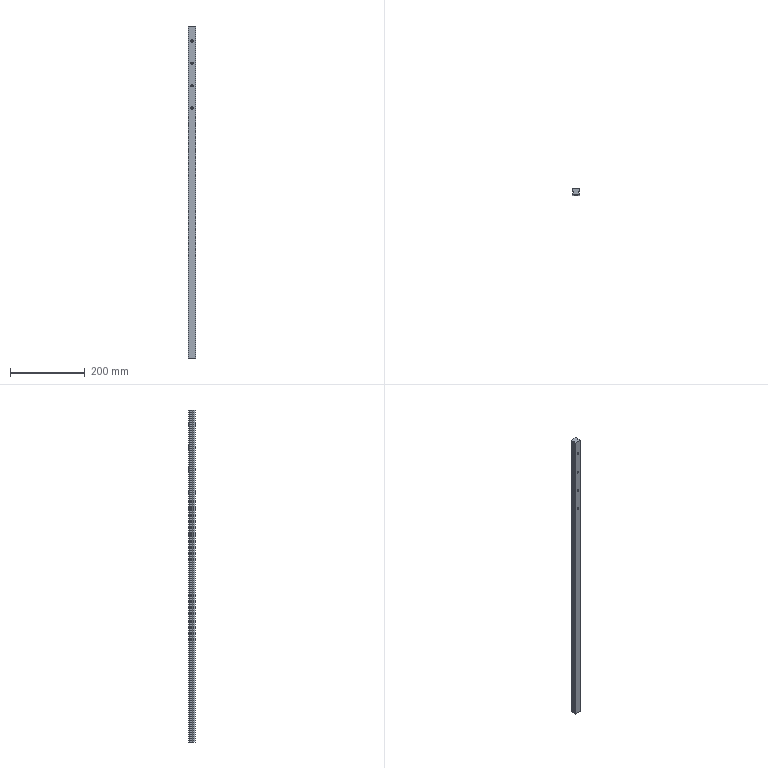Part | SolidWorks | features ICE 15, Chamfer 3, Extrusion 3, Fillet 3, MirrorPattern 3, MirrorSolid 3, RevCut 3, LPattern 2, DeleteBody 1, Dome 1 | 1 solid | 46 faces | box 20 x 17.5 x 890 mm | volume 276758 mm3 | plane 24 | cylinder 22 | commonest cylinder face diameters 6 x8 9.5 x8 1.817 x6
STEP:
#1=CARTESIAN_POINT('',(0.,4.7,228.));
#2=VERTEX_POINT('',#1);
#3=CARTESIAN_POINT('',(0.,4.7,222.));
#4=VERTEX_POINT('',#3);
#5=CARTESIAN_POINT('',(0.,4.7,225.));
#6=DIRECTION('',(0.,-1.,0.));
#7=DIRECTION('',(0.,0.,-1.));
#8=AXIS2_PLACEMENT_3D('',#5,#6,#7);
#9=CIRCLE('',#8,3.);
#10=EDGE_CURVE('',#2,#4,#9,.T.);
#11=ORIENTED_EDGE('',*,*,#10,.F.);
#12=CARTESIAN_POINT('',(0.,-4.3,228.));
#13=VERTEX_POINT('',#12);
#14=CARTESIAN_POINT('',(0.,-4.3,228.));
#15=DIRECTION('',(0.,-1.,0.));
#16=VECTOR('',#15,1000.);
#17=LINE('',#14,#16);
#18=EDGE_CURVE('',#2,#13,#17,.T.);
#19=ORIENTED_EDGE('',*,*,#18,.T.);
#20=CARTESIAN_POINT('',(0.,-4.3,222.));
#21=VERTEX_POINT('',#20);
#22=CARTESIAN_POINT('',(0.,-4.3,225.));
#23=DIRECTION('',(0.,-1.,0.));
#24=DIRECTION('',(0.,0.,-1.));
#25=AXIS2_PLACEMENT_3D('',#22,#23,#24);
#26=CIRCLE('',#25,3.);
#27=EDGE_CURVE('',#13,#21,#26,.T.);
#28=ORIENTED_EDGE('',*,*,#27,.T.);
#29=CARTESIAN_POINT('',(0.,-4.3,222.));
#30=DIRECTION('',(0.,-1.,0.));
#31=VECTOR('',#30,1000.);
#32=LINE('',#29,#31);
#33=EDGE_CURVE('',#4,#21,#32,.T.);
#34=ORIENTED_EDGE('',*,*,#33,.F.);
#35=EDGE_LOOP('',(#11,#19,#28,#34));
#36=FACE_OUTER_BOUND('',#35,.T.);
#37=CARTESIAN_POINT('',(0.,-4.3,225.));
#38=DIRECTION('',(0.,-1.,0.));
#39=DIRECTION('',(0.,0.,-1.));
#40=AXIS2_PLACEMENT_3D('',#37,#38,#39);
#41=CYLINDRICAL_SURFACE('',#40,3.);
#42=ADVANCED_FACE('',(#36),#41,.F.);
#43=CARTESIAN_POINT('',(0.,13.2,229.75));
#44=VERTEX_POINT('',#43);
#45=CARTESIAN_POINT('',(0.,13.2,220.25));
#46=VERTEX_POINT('',#45);
#47=CARTESIAN_POINT('',(0.,13.2,225.));
#48=DIRECTION('',(0.,-1.,0.));
#49=DIRECTION('',(0.,0.,-1.));
#50=AXIS2_PLACEMENT_3D('',#47,#48,#49);
#51=CIRCLE('',#50,4.75);
#52=EDGE_CURVE('',#44,#46,#51,.T.);
#53=ORIENTED_EDGE('',*,*,#52,.F.);
#54=CARTESIAN_POINT('',(0.,4.7,229.75));
#55=VERTEX_POINT('',#54);
#56=CARTESIAN_POINT('',(0.,-4.3,229.75));
#57=DIRECTION('',(0.,-1.,0.));
#58=VECTOR('',#57,1000.);
#59=LINE('',#56,#58);
#60=EDGE_CURVE('',#44,#55,#59,.T.);
#61=ORIENTED_EDGE('',*,*,#60,.T.);
#62=CARTESIAN_POINT('',(0.,4.7,220.25));
#63=VERTEX_POINT('',#62);
#64=CARTESIAN_POINT('',(0.,4.7,225.));
#65=DIRECTION('',(0.,-1.,0.));
#66=DIRECTION('',(0.,0.,-1.));
#67=AXIS2_PLACEMENT_3D('',#64,#65,#66);
#68=CIRCLE('',#67,4.75);
#69=EDGE_CURVE('',#55,#63,#68,.T.);
#70=ORIENTED_EDGE('',*,*,#69,.T.);
#71=CARTESIAN_POINT('',(0.,-4.3,220.25));
#72=DIRECTION('',(0.,-1.,0.));
#73=VECTOR('',#72,1000.);
#74=LINE('',#71,#73);
#75=EDGE_CURVE('',#46,#63,#74,.T.);
#76=ORIENTED_EDGE('',*,*,#75,.F.);
#77=EDGE_LOOP('',(#53,#61,#70,#76));
#78=FACE_OUTER_BOUND('',#77,.T.);
#79=CARTESIAN_POINT('',(0.,-4.3,225.));
#80=DIRECTION('',(0.,-1.,0.));
#81=DIRECTION('',(0.,0.,-1.));
#82=AXIS2_PLACEMENT_3D('',#79,#80,#81);
#83=CYLINDRICAL_SURFACE('',#82,4.75);
#84=ADVANCED_FACE('',(#78),#83,.F.);
#85=CARTESIAN_POINT('',(0.,4.7,288.));
#86=VERTEX_POINT('',#85);
#87=CARTESIAN_POINT('',(0.,4.7,282.));
#88=VERTEX_POINT('',#87);
#89=CARTESIAN_POINT('',(0.,4.7,285.));
#90=DIRECTION('',(0.,-1.,0.));
#91=DIRECTION('',(0.,0.,-1.));
#92=AXIS2_PLACEMENT_3D('',#89,#90,#91);
#93=CIRCLE('',#92,3.);
#94=EDGE_CURVE('',#86,#88,#93,.T.);
#95=ORIENTED_EDGE('',*,*,#94,.F.);
#96=CARTESIAN_POINT('',(0.,-4.3,288.));
#97=VERTEX_POINT('',#96);
#98=CARTESIAN_POINT('',(0.,-4.3,288.));
#99=DIRECTION('',(0.,-1.,0.));
#100=VECTOR('',#99,1000.);
#101=LINE('',#98,#100);
#102=EDGE_CURVE('',#86,#97,#101,.T.);
#103=ORIENTED_EDGE('',*,*,#102,.T.);
#104=CARTESIAN_POINT('',(0.,-4.3,282.));
#105=VERTEX_POINT('',#104);
#106=CARTESIAN_POINT('',(0.,-4.3,285.));
#107=DIRECTION('',(0.,-1.,0.));
#108=DIRECTION('',(0.,0.,-1.));
#109=AXIS2_PLACEMENT_3D('',#106,#107,#108);
#110=CIRCLE('',#109,3.);
#111=EDGE_CURVE('',#97,#105,#110,.T.);
#112=ORIENTED_EDGE('',*,*,#111,.T.);
#113=CARTESIAN_POINT('',(0.,-4.3,282.));
#114=DIRECTION('',(0.,-1.,0.));
#115=VECTOR('',#114,1000.);
#116=LINE('',#113,#115);
#117=EDGE_CURVE('',#88,#105,#116,.T.);
#118=ORIENTED_EDGE('',*,*,#117,.F.);
#119=EDGE_LOOP('',(#95,#103,#112,#118));
#120=FACE_OUTER_BOUND('',#119,.T.);
#121=CARTESIAN_POINT('',(0.,-4.3,285.));
#122=DIRECTION('',(0.,-1.,0.));
#123=DIRECTION('',(0.,0.,-1.));
#124=AXIS2_PLACEMENT_3D('',#121,#122,#123);
#125=CYLINDRICAL_SURFACE('',#124,3.);
#126=ADVANCED_FACE('',(#120),#125,.F.);
#127=CARTESIAN_POINT('',(0.,13.2,289.75));
#128=VERTEX_POINT('',#127);
#129=CARTESIAN_POINT('',(0.,13.2,280.25));
#130=VERTEX_POINT('',#129);
#131=CARTESIAN_POINT('',(0.,13.2,285.));
#132=DIRECTION('',(0.,-1.,0.));
#133=DIRECTION('',(0.,0.,-1.));
#134=AXIS2_PLACEMENT_3D('',#131,#132,#133);
#135=CIRCLE('',#134,4.75);
#136=EDGE_CURVE('',#128,#130,#135,.T.);
#137=ORIENTED_EDGE('',*,*,#136,.F.);
#138=CARTESIAN_POINT('',(0.,4.7,289.75));
#139=VERTEX_POINT('',#138);
#140=CARTESIAN_POINT('',(0.,-4.3,289.75));
#141=DIRECTION('',(0.,-1.,0.));
#142=VECTOR('',#141,1000.);
#143=LINE('',#140,#142);
#144=EDGE_CURVE('',#128,#139,#143,.T.);
#145=ORIENTED_EDGE('',*,*,#144,.T.);
#146=CARTESIAN_POINT('',(0.,4.7,280.25));
#147=VERTEX_POINT('',#146);
#148=CARTESIAN_POINT('',(0.,4.7,285.));
#149=DIRECTION('',(0.,-1.,0.));
#150=DIRECTION('',(0.,0.,-1.));
#151=AXIS2_PLACEMENT_3D('',#148,#149,#150);
#152=CIRCLE('',#151,4.75);
#153=EDGE_CURVE('',#139,#147,#152,.T.);
#154=ORIENTED_EDGE('',*,*,#153,.T.);
#155=CARTESIAN_POINT('',(0.,-4.3,280.25));
#156=DIRECTION('',(0.,-1.,0.));
#157=VECTOR('',#156,1000.);
#158=LINE('',#155,#157);
#159=EDGE_CURVE('',#130,#147,#158,.T.);
#160=ORIENTED_EDGE('',*,*,#159,.F.);
#161=EDGE_LOOP('',(#137,#145,#154,#160));
#162=FACE_OUTER_BOUND('',#161,.T.);
#163=CARTESIAN_POINT('',(0.,-4.3,285.));
#164=DIRECTION('',(0.,-1.,0.));
#165=DIRECTION('',(0.,0.,-1.));
#166=AXIS2_PLACEMENT_3D('',#163,#164,#165);
#167=CYLINDRICAL_SURFACE('',#166,4.75);
#168=ADVANCED_FACE('',(#162),#167,.F.);
#169=CARTESIAN_POINT('',(0.,4.7,348.));
#170=VERTEX_POINT('',#169);
#171=CARTESIAN_POINT('',(0.,4.7,342.));
#172=VERTEX_POINT('',#171);
#173=CARTESIAN_POINT('',(0.,4.7,345.));
#174=DIRECTION('',(0.,-1.,0.));
#175=DIRECTION('',(0.,0.,-1.));
#176=AXIS2_PLACEMENT_3D('',#173,#174,#175);
#177=CIRCLE('',#176,3.);
#178=EDGE_CURVE('',#170,#172,#177,.T.);
#179=ORIENTED_EDGE('',*,*,#178,.F.);
#180=CARTESIAN_POINT('',(0.,-4.3,348.));
#181=VERTEX_POINT('',#180);
#182=CARTESIAN_POINT('',(0.,-4.3,348.));
#183=DIRECTION('',(0.,-1.,0.));
#184=VECTOR('',#183,1000.);
#185=LINE('',#182,#184);
#186=EDGE_CURVE('',#170,#181,#185,.T.);
#187=ORIENTED_EDGE('',*,*,#186,.T.);
#188=CARTESIAN_POINT('',(0.,-4.3,342.));
#189=VERTEX_POINT('',#188);
#190=CARTESIAN_POINT('',(0.,-4.3,345.));
#191=DIRECTION('',(0.,-1.,0.));
#192=DIRECTION('',(0.,0.,-1.));
#193=AXIS2_PLACEMENT_3D('',#190,#191,#192);
#194=CIRCLE('',#193,3.);
#195=EDGE_CURVE('',#181,#189,#194,.T.);
#196=ORIENTED_EDGE('',*,*,#195,.T.);
#197=CARTESIAN_POINT('',(0.,-4.3,342.));
#198=DIRECTION('',(0.,-1.,0.));
#199=VECTOR('',#198,1000.);
#200=LINE('',#197,#199);
#201=EDGE_CURVE('',#172,#189,#200,.T.);
#202=ORIENTED_EDGE('',*,*,#201,.F.);
#203=EDGE_LOOP('',(#179,#187,#196,#202));
#204=FACE_OUTER_BOUND('',#203,.T.);
#205=CARTESIAN_POINT('',(0.,-4.3,345.));
#206=DIRECTION('',(0.,-1.,0.));
#207=DIRECTION('',(0.,0.,-1.));
#208=AXIS2_PLACEMENT_3D('',#205,#206,#207);
#209=CYLINDRICAL_SURFACE('',#208,3.);
#210=ADVANCED_FACE('',(#204),#209,.F.);
#211=CARTESIAN_POINT('',(0.,13.2,349.75));
#212=VERTEX_POINT('',#211);
#213=CARTESIAN_POINT('',(0.,13.2,340.25));
#214=VERTEX_POINT('',#213);
#215=CARTESIAN_POINT('',(0.,13.2,345.));
#216=DIRECTION('',(0.,-1.,0.));
#217=DIRECTION('',(0.,0.,-1.));
#218=AXIS2_PLACEMENT_3D('',#215,#216,#217);
#219=CIRCLE('',#218,4.75);
#220=EDGE_CURVE('',#212,#214,#219,.T.);
#221=ORIENTED_EDGE('',*,*,#220,.F.);
#222=CARTESIAN_POINT('',(0.,4.7,349.75));
#223=VERTEX_POINT('',#222);
#224=CARTESIAN_POINT('',(0.,-4.3,349.75));
#225=DIRECTION('',(0.,-1.,0.));
#226=VECTOR('',#225,1000.);
#227=LINE('',#224,#226);
#228=EDGE_CURVE('',#212,#223,#227,.T.);
#229=ORIENTED_EDGE('',*,*,#228,.T.);
#230=CARTESIAN_POINT('',(0.,4.7,340.25));
#231=VERTEX_POINT('',#230);
#232=CARTESIAN_POINT('',(0.,4.7,345.));
#233=DIRECTION('',(0.,-1.,0.));
#234=DIRECTION('',(0.,0.,-1.));
#235=AXIS2_PLACEMENT_3D('',#232,#233,#234);
#236=CIRCLE('',#235,4.75);
#237=EDGE_CURVE('',#223,#231,#236,.T.);
#238=ORIENTED_EDGE('',*,*,#237,.T.);
#239=CARTESIAN_POINT('',(0.,-4.3,340.25));
#240=DIRECTION('',(0.,-1.,0.));
#241=VECTOR('',#240,1000.);
#242=LINE('',#239,#241);
#243=EDGE_CURVE('',#214,#231,#242,.T.);
#244=ORIENTED_EDGE('',*,*,#243,.F.);
#245=EDGE_LOOP('',(#221,#229,#238,#244));
#246=FACE_OUTER_BOUND('',#245,.T.);
#247=CARTESIAN_POINT('',(0.,-4.3,345.));
#248=DIRECTION('',(0.,-1.,0.));
#249=DIRECTION('',(0.,0.,-1.));
#250=AXIS2_PLACEMENT_3D('',#247,#248,#249);
#251=CYLINDRICAL_SURFACE('',#250,4.75);
#252=ADVANCED_FACE('',(#246),#251,.F.);
#253=CARTESIAN_POINT('',(0.,4.7,408.));
#254=VERTEX_POINT('',#253);
#255=CARTESIAN_POINT('',(0.,4.7,402.));
#256=VERTEX_POINT('',#255);
#257=CARTESIAN_POINT('',(0.,4.7,405.));
#258=DIRECTION('',(0.,-1.,0.));
#259=DIRECTION('',(0.,0.,-1.));
#260=AXIS2_PLACEMENT_3D('',#257,#258,#259);
#261=CIRCLE('',#260,3.);
#262=EDGE_CURVE('',#254,#256,#261,.T.);
#263=ORIENTED_EDGE('',*,*,#262,.F.);
#264=CARTESIAN_POINT('',(0.,-4.3,408.));
#265=VERTEX_POINT('',#264);
#266=CARTESIAN_POINT('',(0.,-4.3,408.));
#267=DIRECTION('',(0.,-1.,0.));
#268=VECTOR('',#267,1000.);
#269=LINE('',#266,#268);
#270=EDGE_CURVE('',#254,#265,#269,.T.);
#271=ORIENTED_EDGE('',*,*,#270,.T.);
#272=CARTESIAN_POINT('',(0.,-4.3,402.));
#273=VERTEX_POINT('',#272);
#274=CARTESIAN_POINT('',(0.,-4.3,405.));
#275=DIRECTION('',(0.,-1.,0.));
#276=DIRECTION('',(0.,0.,-1.));
#277=AXIS2_PLACEMENT_3D('',#274,#275,#276);
#278=CIRCLE('',#277,3.);
#279=EDGE_CURVE('',#265,#273,#278,.T.);
#280=ORIENTED_EDGE('',*,*,#279,.T.);
#281=CARTESIAN_POINT('',(0.,-4.3,402.));
#282=DIRECTION('',(0.,-1.,0.));
#283=VECTOR('',#282,1000.);
#284=LINE('',#281,#283);
#285=EDGE_CURVE('',#256,#273,#284,.T.);
#286=ORIENTED_EDGE('',*,*,#285,.F.);
#287=EDGE_LOOP('',(#263,#271,#280,#286));
#288=FACE_OUTER_BOUND('',#287,.T.);
#289=CARTESIAN_POINT('',(0.,-4.3,405.));
#290=DIRECTION('',(0.,-1.,0.));
#291=DIRECTION('',(0.,0.,-1.));
#292=AXIS2_PLACEMENT_3D('',#289,#290,#291);
#293=CYLINDRICAL_SURFACE('',#292,3.);
#294=ADVANCED_FACE('',(#288),#293,.F.);
#295=CARTESIAN_POINT('',(0.,13.2,409.75));
#296=VERTEX_POINT('',#295);
#297=CARTESIAN_POINT('',(0.,13.2,400.25));
#298=VERTEX_POINT('',#297);
#299=CARTESIAN_POINT('',(0.,13.2,405.));
#300=DIRECTION('',(0.,-1.,0.));
#301=DIRECTION('',(0.,0.,-1.));
#302=AXIS2_PLACEMENT_3D('',#299,#300,#301);
#303=CIRCLE('',#302,4.75);
#304=EDGE_CURVE('',#296,#298,#303,.T.);
#305=ORIENTED_EDGE('',*,*,#304,.F.);
#306=CARTESIAN_POINT('',(0.,4.7,409.75));
#307=VERTEX_POINT('',#306);
#308=CARTESIAN_POINT('',(0.,-4.3,409.75));
#309=DIRECTION('',(0.,-1.,0.));
#310=VECTOR('',#309,1000.);
#311=LINE('',#308,#310);
#312=EDGE_CURVE('',#296,#307,#311,.T.);
#313=ORIENTED_EDGE('',*,*,#312,.T.);
#314=CARTESIAN_POINT('',(0.,4.7,400.25));
#315=VERTEX_POINT('',#314);
#316=CARTESIAN_POINT('',(0.,4.7,405.));
#317=DIRECTION('',(0.,-1.,0.));
#318=DIRECTION('',(0.,0.,-1.));
#319=AXIS2_PLACEMENT_3D('',#316,#317,#318);
#320=CIRCLE('',#319,4.75);
#321=EDGE_CURVE('',#307,#315,#320,.T.);
#322=ORIENTED_EDGE('',*,*,#321,.T.);
#323=CARTESIAN_POINT('',(0.,-4.3,400.25));
#324=DIRECTION('',(0.,-1.,0.));
#325=VECTOR('',#324,1000.);
#326=LINE('',#323,#325);
#327=EDGE_CURVE('',#298,#315,#326,.T.);
#328=ORIENTED_EDGE('',*,*,#327,.F.);
#329=EDGE_LOOP('',(#305,#313,#322,#328));
#330=FACE_OUTER_BOUND('',#329,.T.);
#331=CARTESIAN_POINT('',(0.,-4.3,405.));
#332=DIRECTION('',(0.,-1.,0.));
#333=DIRECTION('',(0.,0.,-1.));
#334=AXIS2_PLACEMENT_3D('',#331,#332,#333);
#335=CYLINDRICAL_SURFACE('',#334,4.75);
#336=ADVANCED_FACE('',(#330),#335,.F.);
#337=CARTESIAN_POINT('',(8.152,12.26,445.));
#338=VERTEX_POINT('',#337);
#339=CARTESIAN_POINT('',(8.152,12.276,445.));
#340=VERTEX_POINT('',#339);
#341=CARTESIAN_POINT('',(9.06,12.26,445.));
#342=DIRECTION('',(0.,0.,-1.));
#343=DIRECTION('',(1.,0.,0.));
#344=AXIS2_PLACEMENT_3D('',#341,#342,#343);
#345=CIRCLE('',#344,0.9086);
#346=EDGE_CURVE('',#338,#340,#345,.T.);
#347=ORIENTED_EDGE('',*,*,#346,.F.);
#348=CARTESIAN_POINT('',(8.152,12.26,-445.));
#349=VERTEX_POINT('',#348);
#350=CARTESIAN_POINT('',(8.152,12.26,445.));
#351=DIRECTION('',(0.,0.,-1.));
#352=VECTOR('',#351,1000.);
#353=LINE('',#350,#352);
#354=EDGE_CURVE('',#338,#349,#353,.T.);
#355=ORIENTED_EDGE('',*,*,#354,.T.);
#356=CARTESIAN_POINT('',(8.152,12.276,-445.));
#357=VERTEX_POINT('',#356);
#358=CARTESIAN_POINT('',(9.06,12.26,-445.));
#359=DIRECTION('',(0.,0.,-1.));
#360=DIRECTION('',(1.,0.,0.));
#361=AXIS2_PLACEMENT_3D('',#358,#359,#360);
#362=CIRCLE('',#361,0.9086);
#363=EDGE_CURVE('',#349,#357,#362,.T.);
#364=ORIENTED_EDGE('',*,*,#363,.T.);
#365=CARTESIAN_POINT('',(8.152,12.276,445.));
#366=DIRECTION('',(0.,0.,-1.));
#367=VECTOR('',#366,1000.);
#368=LINE('',#365,#367);
#369=EDGE_CURVE('',#340,#357,#368,.T.);
#370=ORIENTED_EDGE('',*,*,#369,.F.);
#371=EDGE_LOOP('',(#347,#355,#364,#370));
#372=FACE_OUTER_BOUND('',#371,.T.);
#373=CARTESIAN_POINT('',(9.06,12.26,445.));
#374=DIRECTION('',(0.,0.,-1.));
#375=DIRECTION('',(-1.,0.,0.));
#376=AXIS2_PLACEMENT_3D('',#373,#374,#375);
#377=CYLINDRICAL_SURFACE('',#376,0.9086);
#378=ADVANCED_FACE('',(#372),#377,.F.);
#379=CARTESIAN_POINT('',(8.152,6.22,445.));
#380=VERTEX_POINT('',#379);
#381=CARTESIAN_POINT('',(9.076,7.128,445.));
#382=VERTEX_POINT('',#381);
#383=CARTESIAN_POINT('',(9.06,6.22,445.));
#384=DIRECTION('',(0.,0.,-1.));
#385=DIRECTION('',(1.,0.,0.));
#386=AXIS2_PLACEMENT_3D('',#383,#384,#385);
#387=CIRCLE('',#386,0.9086);
#388=EDGE_CURVE('',#380,#382,#387,.T.);
#389=ORIENTED_EDGE('',*,*,#388,.F.);
#390=CARTESIAN_POINT('',(8.152,6.22,-445.));
#391=VERTEX_POINT('',#390);
#392=CARTESIAN_POINT('',(8.152,6.22,445.));
#393=DIRECTION('',(0.,0.,-1.));
#394=VECTOR('',#393,1000.);
#395=LINE('',#392,#394);
#396=EDGE_CURVE('',#380,#391,#395,.T.);
#397=ORIENTED_EDGE('',*,*,#396,.T.);
#398=CARTESIAN_POINT('',(9.076,7.128,-445.));
#399=VERTEX_POINT('',#398);
#400=CARTESIAN_POINT('',(9.06,6.22,-445.));
#401=DIRECTION('',(0.,0.,-1.));
#402=DIRECTION('',(1.,0.,0.));
#403=AXIS2_PLACEMENT_3D('',#400,#401,#402);
#404=CIRCLE('',#403,0.9086);
#405=EDGE_CURVE('',#391,#399,#404,.T.);
#406=ORIENTED_EDGE('',*,*,#405,.T.);
#407=CARTESIAN_POINT('',(9.076,7.128,445.));
#408=DIRECTION('',(0.,0.,-1.));
#409=VECTOR('',#408,1000.);
#410=LINE('',#407,#409);
#411=EDGE_CURVE('',#382,#399,#410,.T.);
#412=ORIENTED_EDGE('',*,*,#411,.F.);
#413=EDGE_LOOP('',(#389,#397,#406,#412));
#414=FACE_OUTER_BOUND('',#413,.T.);
#415=CARTESIAN_POINT('',(9.06,6.22,445.));
#416=DIRECTION('',(0.,0.,-1.));
#417=DIRECTION('',(-1.,0.,0.));
#418=AXIS2_PLACEMENT_3D('',#415,#416,#417);
#419=CYLINDRICAL_SURFACE('',#418,0.9086);
#420=ADVANCED_FACE('',(#414),#419,.F.);
#421=ORIENTED_EDGE('',*,*,#369,.T.);
#422=CARTESIAN_POINT('',(7.228,13.2,-445.));
#423=VERTEX_POINT('',#422);
#424=CARTESIAN_POINT('',(8.152,12.276,-445.));
#425=DIRECTION('',(-0.7071,0.7071,0.));
#426=VECTOR('',#425,1000.);
#427=LINE('',#424,#426);
#428=EDGE_CURVE('',#357,#423,#427,.T.);
#429=ORIENTED_EDGE('',*,*,#428,.T.);
#430=CARTESIAN_POINT('',(7.228,13.2,445.));
#431=VERTEX_POINT('',#430);
#432=CARTESIAN_POINT('',(7.228,13.2,445.));
#433=DIRECTION('',(0.,0.,-1.));
#434=VECTOR('',#433,1000.);
#435=LINE('',#432,#434);
#436=EDGE_CURVE('',#431,#423,#435,.T.);
#437=ORIENTED_EDGE('',*,*,#436,.F.);
#438=CARTESIAN_POINT('',(8.152,12.276,445.));
#439=DIRECTION('',(-0.7071,0.7071,0.));
#440=VECTOR('',#439,1000.);
#441=LINE('',#438,#440);
#442=EDGE_CURVE('',#340,#431,#441,.T.);
#443=ORIENTED_EDGE('',*,*,#442,.F.);
#444=EDGE_LOOP('',(#421,#429,#437,#443));
#445=FACE_OUTER_BOUND('',#444,.T.);
#446=CARTESIAN_POINT('',(8.152,12.276,445.));
#447=DIRECTION('',(-0.7071,-0.7071,0.));
#448=DIRECTION('',(0.7071,-0.7071,0.));
#449=AXIS2_PLACEMENT_3D('',#446,#447,#448);
#450=PLANE('',#449);
#451=ADVANCED_FACE('',(#445),#450,.F.);
#452=CARTESIAN_POINT('',(0.,13.2,225.));
#453=DIRECTION('',(0.,-1.,0.));
#454=DIRECTION('',(0.,0.,-1.));
#455=AXIS2_PLACEMENT_3D('',#452,#453,#454);
#456=CIRCLE('',#455,4.75);
#457=EDGE_CURVE('',#46,#44,#456,.T.);
#458=ORIENTED_EDGE('',*,*,#457,.T.);
#459=ORIENTED_EDGE('',*,*,#52,.T.);
#460=EDGE_LOOP('',(#458,#459));
#461=FACE_BOUND('',#460,.T.);
#462=CARTESIAN_POINT('',(0.,13.2,285.));
#463=DIRECTION('',(0.,-1.,0.));
#464=DIRECTION('',(0.,0.,-1.));
#465=AXIS2_PLACEMENT_3D('',#462,#463,#464);
#466=CIRCLE('',#465,4.75);
#467=EDGE_CURVE('',#130,#128,#466,.T.);
#468=ORIENTED_EDGE('',*,*,#467,.T.);
#469=ORIENTED_EDGE('',*,*,#136,.T.);
#470=EDGE_LOOP('',(#468,#469));
#471=FACE_BOUND('',#470,.T.);
#472=CARTESIAN_POINT('',(0.,13.2,345.));
#473=DIRECTION('',(0.,-1.,0.));
#474=DIRECTION('',(0.,0.,-1.));
#475=AXIS2_PLACEMENT_3D('',#472,#473,#474);
#476=CIRCLE('',#475,4.75);
#477=EDGE_CURVE('',#214,#212,#476,.T.);
#478=ORIENTED_EDGE('',*,*,#477,.T.);
#479=ORIENTED_EDGE('',*,*,#220,.T.);
#480=EDGE_LOOP('',(#478,#479));
#481=FACE_BOUND('',#480,.T.);
#482=CARTESIAN_POINT('',(0.,13.2,405.));
#483=DIRECTION('',(0.,-1.,0.));
#484=DIRECTION('',(0.,0.,-1.));
#485=AXIS2_PLACEMENT_3D('',#482,#483,#484);
#486=CIRCLE('',#485,4.75);
#487=EDGE_CURVE('',#298,#296,#486,.T.);
#488=ORIENTED_EDGE('',*,*,#487,.T.);
#489=ORIENTED_EDGE('',*,*,#304,.T.);
#490=EDGE_LOOP('',(#488,#489));
#491=FACE_BOUND('',#490,.T.);
#492=ORIENTED_EDGE('',*,*,#436,.T.);
#493=CARTESIAN_POINT('',(-7.228,13.2,-445.));
#494=VERTEX_POINT('',#493);
#495=CARTESIAN_POINT('',(7.228,13.2,-445.));
#496=DIRECTION('',(-1.,0.,0.));
#497=VECTOR('',#496,1000.);
#498=LINE('',#495,#497);
#499=EDGE_CURVE('',#423,#494,#498,.T.);
#500=ORIENTED_EDGE('',*,*,#499,.T.);
#501=CARTESIAN_POINT('',(-7.228,13.2,445.));
#502=VERTEX_POINT('',#501);
#503=CARTESIAN_POINT('',(-7.228,13.2,445.));
#504=DIRECTION('',(0.,0.,-1.));
#505=VECTOR('',#504,1000.);
#506=LINE('',#503,#505);
#507=EDGE_CURVE('',#502,#494,#506,.T.);
#508=ORIENTED_EDGE('',*,*,#507,.F.);
#509=CARTESIAN_POINT('',(7.228,13.2,445.));
#510=DIRECTION('',(-1.,0.,0.));
#511=VECTOR('',#510,1000.);
#512=LINE('',#509,#511);
#513=EDGE_CURVE('',#431,#502,#512,.T.);
#514=ORIENTED_EDGE('',*,*,#513,.F.);
#515=EDGE_LOOP('',(#492,#500,#508,#514));
#516=FACE_OUTER_BOUND('',#515,.T.);
#517=CARTESIAN_POINT('',(7.228,13.2,445.));
#518=DIRECTION('',(0.,-1.,0.));
#519=DIRECTION('',(0.,0.,-1.));
#520=AXIS2_PLACEMENT_3D('',#517,#518,#519);
#521=PLANE('',#520);
#522=ADVANCED_FACE('',(#461,#471,#481,#491,#516),#521,.F.);
#523=ORIENTED_EDGE('',*,*,#507,.T.);
#524=CARTESIAN_POINT('',(-8.152,12.276,-445.));
#525=VERTEX_POINT('',#524);
#526=CARTESIAN_POINT('',(-8.152,12.276,-445.));
#527=DIRECTION('',(-0.7071,-0.7071,0.));
#528=VECTOR('',#527,1000.);
#529=LINE('',#526,#528);
#530=EDGE_CURVE('',#494,#525,#529,.T.);
#531=ORIENTED_EDGE('',*,*,#530,.T.);
#532=CARTESIAN_POINT('',(-8.152,12.276,445.));
#533=VERTEX_POINT('',#532);
#534=CARTESIAN_POINT('',(-8.152,12.276,445.));
#535=DIRECTION('',(0.,0.,-1.));
#536=VECTOR('',#535,1000.);
#537=LINE('',#534,#536);
#538=EDGE_CURVE('',#533,#525,#537,.T.);
#539=ORIENTED_EDGE('',*,*,#538,.F.);
#540=CARTESIAN_POINT('',(-8.152,12.276,445.));
#541=DIRECTION('',(-0.7071,-0.7071,0.));
#542=VECTOR('',#541,1000.);
#543=LINE('',#540,#542);
#544=EDGE_CURVE('',#502,#533,#543,.T.);
#545=ORIENTED_EDGE('',*,*,#544,.F.);
#546=EDGE_LOOP('',(#523,#531,#539,#545));
#547=FACE_OUTER_BOUND('',#546,.T.);
#548=CARTESIAN_POINT('',(-8.152,12.276,445.));
#549=DIRECTION('',(0.7071,-0.7071,0.));
#550=DIRECTION('',(0.7071,0.7071,0.));
#551=AXIS2_PLACEMENT_3D('',#548,#549,#550);
#552=PLANE('',#551);
#553=ADVANCED_FACE('',(#547),#552,.F.);
#554=ORIENTED_EDGE('',*,*,#538,.T.);
#555=CARTESIAN_POINT('',(-9.076,11.352,-445.));
#556=VERTEX_POINT('',#555);
#557=CARTESIAN_POINT('',(-9.06,12.26,-445.));
#558=DIRECTION('',(0.,0.,-1.));
#559=DIRECTION('',(1.,0.,0.));
#560=AXIS2_PLACEMENT_3D('',#557,#558,#559);
#561=CIRCLE('',#560,0.9086);
#562=EDGE_CURVE('',#525,#556,#561,.T.);
#563=ORIENTED_EDGE('',*,*,#562,.T.);
#564=CARTESIAN_POINT('',(-9.076,11.352,445.));
#565=VERTEX_POINT('',#564);
#566=CARTESIAN_POINT('',(-9.076,11.352,445.));
#567=DIRECTION('',(0.,0.,-1.));
#568=VECTOR('',#567,1000.);
#569=LINE('',#566,#568);
#570=EDGE_CURVE('',#565,#556,#569,.T.);
#571=ORIENTED_EDGE('',*,*,#570,.F.);
#572=CARTESIAN_POINT('',(-9.06,12.26,445.));
#573=DIRECTION('',(0.,0.,-1.));
#574=DIRECTION('',(1.,0.,0.));
#575=AXIS2_PLACEMENT_3D('',#572,#573,#574);
#576=CIRCLE('',#575,0.9086);
#577=EDGE_CURVE('',#533,#565,#576,.T.);
#578=ORIENTED_EDGE('',*,*,#577,.F.);
#579=EDGE_LOOP('',(#554,#563,#571,#578));
#580=FACE_OUTER_BOUND('',#579,.T.);
#581=CARTESIAN_POINT('',(-9.06,12.26,445.));
#582=DIRECTION('',(0.,0.,-1.));
#583=DIRECTION('',(-1.,0.,0.));
#584=AXIS2_PLACEMENT_3D('',#581,#582,#583);
#585=CYLINDRICAL_SURFACE('',#584,0.9086);
#586=ADVANCED_FACE('',(#580),#585,.F.);
#587=ORIENTED_EDGE('',*,*,#570,.T.);
#588=CARTESIAN_POINT('',(-10.,10.428,-445.));
#589=VERTEX_POINT('',#588);
#590=CARTESIAN_POINT('',(-10.,10.428,-445.));
#591=DIRECTION('',(-0.7071,-0.7071,0.));
#592=VECTOR('',#591,1000.);
#593=LINE('',#590,#592);
#594=EDGE_CURVE('',#556,#589,#593,.T.);
#595=ORIENTED_EDGE('',*,*,#594,.T.);
#596=CARTESIAN_POINT('',(-10.,10.428,445.));
#597=VERTEX_POINT('',#596);
#598=CARTESIAN_POINT('',(-10.,10.428,445.));
#599=DIRECTION('',(0.,0.,-1.));
#600=VECTOR('',#599,1000.);
#601=LINE('',#598,#600);
#602=EDGE_CURVE('',#597,#589,#601,.T.);
#603=ORIENTED_EDGE('',*,*,#602,.F.);
#604=CARTESIAN_POINT('',(-10.,10.428,445.));
#605=DIRECTION('',(-0.7071,-0.7071,0.));
#606=VECTOR('',#605,1000.);
#607=LINE('',#604,#606);
#608=EDGE_CURVE('',#565,#597,#607,.T.);
#609=ORIENTED_EDGE('',*,*,#608,.F.);
#610=EDGE_LOOP('',(#587,#595,#603,#609));
#611=FACE_OUTER_BOUND('',#610,.T.);
#612=CARTESIAN_POINT('',(-10.,10.428,445.));
#613=DIRECTION('',(0.7071,-0.7071,0.));
#614=DIRECTION('',(0.7071,0.7071,0.));
#615=AXIS2_PLACEMENT_3D('',#612,#613,#614);
#616=PLANE('',#615);
#617=ADVANCED_FACE('',(#611),#616,.F.);
#618=ORIENTED_EDGE('',*,*,#602,.T.);
#619=CARTESIAN_POINT('',(-10.,8.052,-445.));
#620=VERTEX_POINT('',#619);
#621=CARTESIAN_POINT('',(-10.,8.052,-445.));
#622=DIRECTION('',(0.,-1.,0.));
#623=VECTOR('',#622,1000.);
#624=LINE('',#621,#623);
#625=EDGE_CURVE('',#589,#620,#624,.T.);
#626=ORIENTED_EDGE('',*,*,#625,.T.);
#627=CARTESIAN_POINT('',(-10.,8.052,445.));
#628=VERTEX_POINT('',#627);
#629=CARTESIAN_POINT('',(-10.,8.052,445.));
#630=DIRECTION('',(0.,0.,-1.));
#631=VECTOR('',#630,1000.);
#632=LINE('',#629,#631);
#633=EDGE_CURVE('',#628,#620,#632,.T.);
#634=ORIENTED_EDGE('',*,*,#633,.F.);
#635=CARTESIAN_POINT('',(-10.,8.052,445.));
#636=DIRECTION('',(0.,-1.,0.));
#637=VECTOR('',#636,1000.);
#638=LINE('',#635,#637);
#639=EDGE_CURVE('',#597,#628,#638,.T.);
#640=ORIENTED_EDGE('',*,*,#639,.F.);
#641=EDGE_LOOP('',(#618,#626,#634,#640));
#642=FACE_OUTER_BOUND('',#641,.T.);
#643=CARTESIAN_POINT('',(-10.,8.052,445.));
#644=DIRECTION('',(1.,0.,0.));
#645=DIRECTION('',(0.,1.,0.));
#646=AXIS2_PLACEMENT_3D('',#643,#644,#645);
#647=PLANE('',#646);
#648=ADVANCED_FACE('',(#642),#647,.F.);
#649=ORIENTED_EDGE('',*,*,#633,.T.);
#650=CARTESIAN_POINT('',(-9.076,7.128,-445.));
#651=VERTEX_POINT('',#650);
#652=CARTESIAN_POINT('',(-9.076,7.128,-445.));
#653=DIRECTION('',(0.7071,-0.7071,0.));
#654=VECTOR('',#653,1000.);
#655=LINE('',#652,#654);
#656=EDGE_CURVE('',#620,#651,#655,.T.);
#657=ORIENTED_EDGE('',*,*,#656,.T.);
#658=CARTESIAN_POINT('',(-9.076,7.128,445.));
#659=VERTEX_POINT('',#658);
#660=CARTESIAN_POINT('',(-9.076,7.128,445.));
#661=DIRECTION('',(0.,0.,-1.));
#662=VECTOR('',#661,1000.);
#663=LINE('',#660,#662);
#664=EDGE_CURVE('',#659,#651,#663,.T.);
#665=ORIENTED_EDGE('',*,*,#664,.F.);
#666=CARTESIAN_POINT('',(-9.076,7.128,445.));
#667=DIRECTION('',(0.7071,-0.7071,0.));
#668=VECTOR('',#667,1000.);
#669=LINE('',#666,#668);
#670=EDGE_CURVE('',#628,#659,#669,.T.);
#671=ORIENTED_EDGE('',*,*,#670,.F.);
#672=EDGE_LOOP('',(#649,#657,#665,#671));
#673=FACE_OUTER_BOUND('',#672,.T.);
#674=CARTESIAN_POINT('',(-9.076,7.128,445.));
#675=DIRECTION('',(0.7071,0.7071,0.));
#676=DIRECTION('',(-0.7071,0.7071,0.));
#677=AXIS2_PLACEMENT_3D('',#674,#675,#676);
#678=PLANE('',#677);
#679=ADVANCED_FACE('',(#673),#678,.F.);
#680=ORIENTED_EDGE('',*,*,#664,.T.);
#681=CARTESIAN_POINT('',(-8.152,6.204,-445.));
#682=VERTEX_POINT('',#681);
#683=CARTESIAN_POINT('',(-9.06,6.22,-445.));
#684=DIRECTION('',(0.,0.,-1.));
#685=DIRECTION('',(1.,0.,0.));
#686=AXIS2_PLACEMENT_3D('',#683,#684,#685);
#687=CIRCLE('',#686,0.9086);
#688=EDGE_CURVE('',#651,#682,#687,.T.);
#689=ORIENTED_EDGE('',*,*,#688,.T.);
#690=CARTESIAN_POINT('',(-8.152,6.204,445.));
#691=VERTEX_POINT('',#690);
#692=CARTESIAN_POINT('',(-8.152,6.204,445.));
#693=DIRECTION('',(0.,0.,-1.));
#694=VECTOR('',#693,1000.);
#695=LINE('',#692,#694);
#696=EDGE_CURVE('',#691,#682,#695,.T.);
#697=ORIENTED_EDGE('',*,*,#696,.F.);
#698=CARTESIAN_POINT('',(-9.06,6.22,445.));
#699=DIRECTION('',(0.,0.,-1.));
#700=DIRECTION('',(1.,0.,0.));
#701=AXIS2_PLACEMENT_3D('',#698,#699,#700);
#702=CIRCLE('',#701,0.9086);
#703=EDGE_CURVE('',#659,#691,#702,.T.);
#704=ORIENTED_EDGE('',*,*,#703,.F.);
#705=EDGE_LOOP('',(#680,#689,#697,#704));
#706=FACE_OUTER_BOUND('',#705,.T.);
#707=CARTESIAN_POINT('',(-9.06,6.22,445.));
#708=DIRECTION('',(0.,0.,-1.));
#709=DIRECTION('',(-1.,0.,0.));
#710=AXIS2_PLACEMENT_3D('',#707,#708,#709);
#711=CYLINDRICAL_SURFACE('',#710,0.9086);
#712=ADVANCED_FACE('',(#706),#711,.F.);
#713=ORIENTED_EDGE('',*,*,#696,.T.);
#714=CARTESIAN_POINT('',(-7.228,5.28,-445.));
#715=VERTEX_POINT('',#714);
#716=CARTESIAN_POINT('',(-7.228,5.28,-445.));
#717=DIRECTION('',(0.7071,-0.7071,0.));
#718=VECTOR('',#717,1000.);
#719=LINE('',#716,#718);
#720=EDGE_CURVE('',#682,#715,#719,.T.);
#721=ORIENTED_EDGE('',*,*,#720,.T.);
#722=CARTESIAN_POINT('',(-7.228,5.28,445.));
#723=VERTEX_POINT('',#722);
#724=CARTESIAN_POINT('',(-7.228,5.28,445.));
#725=DIRECTION('',(0.,0.,-1.));
#726=VECTOR('',#725,1000.);
#727=LINE('',#724,#726);
#728=EDGE_CURVE('',#723,#715,#727,.T.);
#729=ORIENTED_EDGE('',*,*,#728,.F.);
#730=CARTESIAN_POINT('',(-7.228,5.28,445.));
#731=DIRECTION('',(0.7071,-0.7071,0.));
#732=VECTOR('',#731,1000.);
#733=LINE('',#730,#732);
#734=EDGE_CURVE('',#691,#723,#733,.T.);
#735=ORIENTED_EDGE('',*,*,#734,.F.);
#736=EDGE_LOOP('',(#713,#721,#729,#735));
#737=FACE_OUTER_BOUND('',#736,.T.);
#738=CARTESIAN_POINT('',(-7.228,5.28,445.));
#739=DIRECTION('',(0.7071,0.7071,0.));
#740=DIRECTION('',(-0.7071,0.7071,0.));
#741=AXIS2_PLACEMENT_3D('',#738,#739,#740);
#742=PLANE('',#741);
#743=ADVANCED_FACE('',(#737),#742,.F.);
#744=ORIENTED_EDGE('',*,*,#728,.T.);
#745=CARTESIAN_POINT('',(-7.228,3.272,-445.));
#746=VERTEX_POINT('',#745);
#747=CARTESIAN_POINT('',(-7.228,3.272,-445.));
#748=DIRECTION('',(0.,-1.,0.));
#749=VECTOR('',#748,1000.);
#750=LINE('',#747,#749);
#751=EDGE_CURVE('',#715,#746,#750,.T.);
#752=ORIENTED_EDGE('',*,*,#751,.T.);
#753=CARTESIAN_POINT('',(-7.228,3.272,445.));
#754=VERTEX_POINT('',#753);
#755=CARTESIAN_POINT('',(-7.228,3.272,445.));
#756=DIRECTION('',(0.,0.,-1.));
#757=VECTOR('',#756,1000.);
#758=LINE('',#755,#757);
#759=EDGE_CURVE('',#754,#746,#758,.T.);
#760=ORIENTED_EDGE('',*,*,#759,.F.);
#761=CARTESIAN_POINT('',(-7.228,3.272,445.));
#762=DIRECTION('',(0.,-1.,0.));
#763=VECTOR('',#762,1000.);
#764=LINE('',#761,#763);
#765=EDGE_CURVE('',#723,#754,#764,.T.);
#766=ORIENTED_EDGE('',*,*,#765,.F.);
#767=EDGE_LOOP('',(#744,#752,#760,#766));
#768=FACE_OUTER_BOUND('',#767,.T.);
#769=CARTESIAN_POINT('',(-7.228,3.272,445.));
#770=DIRECTION('',(1.,0.,0.));
#771=DIRECTION('',(0.,1.,0.));
#772=AXIS2_PLACEMENT_3D('',#769,#770,#771);
#773=PLANE('',#772);
#774=ADVANCED_FACE('',(#768),#773,.F.);
#775=ORIENTED_EDGE('',*,*,#759,.T.);
#776=CARTESIAN_POINT('',(-10.,0.5,-445.));
#777=VERTEX_POINT('',#776);
#778=CARTESIAN_POINT('',(-10.,0.5,-445.));
#779=DIRECTION('',(-0.7071,-0.7071,0.));
#780=VECTOR('',#779,1000.);
#781=LINE('',#778,#780);
#782=EDGE_CURVE('',#746,#777,#781,.T.);
#783=ORIENTED_EDGE('',*,*,#782,.T.);
#784=CARTESIAN_POINT('',(-10.,0.5,445.));
#785=VERTEX_POINT('',#784);
#786=CARTESIAN_POINT('',(-10.,0.5,445.));
#787=DIRECTION('',(0.,0.,-1.));
#788=VECTOR('',#787,1000.);
#789=LINE('',#786,#788);
#790=EDGE_CURVE('',#785,#777,#789,.T.);
#791=ORIENTED_EDGE('',*,*,#790,.F.);
#792=CARTESIAN_POINT('',(-10.,0.5,445.));
#793=DIRECTION('',(-0.7071,-0.7071,0.));
#794=VECTOR('',#793,1000.);
#795=LINE('',#792,#794);
#796=EDGE_CURVE('',#754,#785,#795,.T.);
#797=ORIENTED_EDGE('',*,*,#796,.F.);
#798=EDGE_LOOP('',(#775,#783,#791,#797));
#799=FACE_OUTER_BOUND('',#798,.T.);
#800=CARTESIAN_POINT('',(-10.,0.5,445.));
#801=DIRECTION('',(0.7071,-0.7071,0.));
#802=DIRECTION('',(0.7071,0.7071,0.));
#803=AXIS2_PLACEMENT_3D('',#800,#801,#802);
#804=PLANE('',#803);
#805=ADVANCED_FACE('',(#799),#804,.F.);
#806=ORIENTED_EDGE('',*,*,#790,.T.);
#807=CARTESIAN_POINT('',(-10.,-4.3,-445.));
#808=VERTEX_POINT('',#807);
#809=CARTESIAN_POINT('',(-10.,-4.3,-445.));
#810=DIRECTION('',(0.,-1.,0.));
#811=VECTOR('',#810,1000.);
#812=LINE('',#809,#811);
#813=EDGE_CURVE('',#777,#808,#812,.T.);
#814=ORIENTED_EDGE('',*,*,#813,.T.);
#815=CARTESIAN_POINT('',(-10.,-4.3,445.));
#816=VERTEX_POINT('',#815);
#817=CARTESIAN_POINT('',(-10.,-4.3,445.));
#818=DIRECTION('',(0.,0.,-1.));
#819=VECTOR('',#818,1000.);
#820=LINE('',#817,#819);
#821=EDGE_CURVE('',#816,#808,#820,.T.);
#822=ORIENTED_EDGE('',*,*,#821,.F.);
#823=CARTESIAN_POINT('',(-10.,-4.3,445.));
#824=DIRECTION('',(0.,-1.,0.));
#825=VECTOR('',#824,1000.);
#826=LINE('',#823,#825);
#827=EDGE_CURVE('',#785,#816,#826,.T.);
#828=ORIENTED_EDGE('',*,*,#827,.F.);
#829=EDGE_LOOP('',(#806,#814,#822,#828));
#830=FACE_OUTER_BOUND('',#829,.T.);
#831=CARTESIAN_POINT('',(-10.,-4.3,445.));
#832=DIRECTION('',(1.,0.,0.));
#833=DIRECTION('',(0.,1.,0.));
#834=AXIS2_PLACEMENT_3D('',#831,#832,#833);
#835=PLANE('',#834);
#836=ADVANCED_FACE('',(#830),#835,.F.);
#837=CARTESIAN_POINT('',(0.,-4.3,225.));
#838=DIRECTION('',(0.,-1.,0.));
#839=DIRECTION('',(0.,0.,-1.));
#840=AXIS2_PLACEMENT_3D('',#837,#838,#839);
#841=CIRCLE('',#840,3.);
#842=EDGE_CURVE('',#21,#13,#841,.T.);
#843=ORIENTED_EDGE('',*,*,#842,.F.);
#844=ORIENTED_EDGE('',*,*,#27,.F.);
#845=EDGE_LOOP('',(#843,#844));
#846=FACE_BOUND('',#845,.T.);
#847=CARTESIAN_POINT('',(0.,-4.3,285.));
#848=DIRECTION('',(0.,-1.,0.));
#849=DIRECTION('',(0.,0.,-1.));
#850=AXIS2_PLACEMENT_3D('',#847,#848,#849);
#851=CIRCLE('',#850,3.);
#852=EDGE_CURVE('',#105,#97,#851,.T.);
#853=ORIENTED_EDGE('',*,*,#852,.F.);
#854=ORIENTED_EDGE('',*,*,#111,.F.);
#855=EDGE_LOOP('',(#853,#854));
#856=FACE_BOUND('',#855,.T.);
#857=CARTESIAN_POINT('',(0.,-4.3,345.));
#858=DIRECTION('',(0.,-1.,0.));
#859=DIRECTION('',(0.,0.,-1.));
#860=AXIS2_PLACEMENT_3D('',#857,#858,#859);
#861=CIRCLE('',#860,3.);
#862=EDGE_CURVE('',#189,#181,#861,.T.);
#863=ORIENTED_EDGE('',*,*,#862,.F.);
#864=ORIENTED_EDGE('',*,*,#195,.F.);
#865=EDGE_LOOP('',(#863,#864));
#866=FACE_BOUND('',#865,.T.);
#867=CARTESIAN_POINT('',(0.,-4.3,405.));
#868=DIRECTION('',(0.,-1.,0.));
#869=DIRECTION('',(0.,0.,-1.));
#870=AXIS2_PLACEMENT_3D('',#867,#868,#869);
#871=CIRCLE('',#870,3.);
#872=EDGE_CURVE('',#273,#265,#871,.T.);
#873=ORIENTED_EDGE('',*,*,#872,.F.);
#874=ORIENTED_EDGE('',*,*,#279,.F.);
#875=EDGE_LOOP('',(#873,#874));
#876=FACE_BOUND('',#875,.T.);
#877=ORIENTED_EDGE('',*,*,#821,.T.);
#878=CARTESIAN_POINT('',(10.,-4.3,-445.));
#879=VERTEX_POINT('',#878);
#880=CARTESIAN_POINT('',(-10.,-4.3,-445.));
#881=DIRECTION('',(1.,0.,0.));
#882=VECTOR('',#881,1000.);
#883=LINE('',#880,#882);
#884=EDGE_CURVE('',#808,#879,#883,.T.);
#885=ORIENTED_EDGE('',*,*,#884,.T.);
#886=CARTESIAN_POINT('',(10.,-4.3,445.));
#887=VERTEX_POINT('',#886);
#888=CARTESIAN_POINT('',(10.,-4.3,445.));
#889=DIRECTION('',(0.,0.,-1.));
#890=VECTOR('',#889,1000.);
#891=LINE('',#888,#890);
#892=EDGE_CURVE('',#887,#879,#891,.T.);
#893=ORIENTED_EDGE('',*,*,#892,.F.);
#894=CARTESIAN_POINT('',(-10.,-4.3,445.));
#895=DIRECTION('',(1.,0.,0.));
#896=VECTOR('',#895,1000.);
#897=LINE('',#894,#896);
#898=EDGE_CURVE('',#816,#887,#897,.T.);
#899=ORIENTED_EDGE('',*,*,#898,.F.);
#900=EDGE_LOOP('',(#877,#885,#893,#899));
#901=FACE_OUTER_BOUND('',#900,.T.);
#902=CARTESIAN_POINT('',(-10.,-4.3,445.));
#903=DIRECTION('',(0.,1.,0.));
#904=DIRECTION('',(0.,0.,1.));
#905=AXIS2_PLACEMENT_3D('',#902,#903,#904);
#906=PLANE('',#905);
#907=ADVANCED_FACE('',(#846,#856,#866,#876,#901),#906,.F.);
#908=ORIENTED_EDGE('',*,*,#892,.T.);
#909=CARTESIAN_POINT('',(10.,0.5,-445.));
#910=VERTEX_POINT('',#909);
#911=CARTESIAN_POINT('',(10.,-4.3,-445.));
#912=DIRECTION('',(0.,1.,0.));
#913=VECTOR('',#912,1000.);
#914=LINE('',#911,#913);
#915=EDGE_CURVE('',#879,#910,#914,.T.);
#916=ORIENTED_EDGE('',*,*,#915,.T.);
#917=CARTESIAN_POINT('',(10.,0.5,445.));
#918=VERTEX_POINT('',#917);
#919=CARTESIAN_POINT('',(10.,0.5,445.));
#920=DIRECTION('',(0.,0.,-1.));
#921=VECTOR('',#920,1000.);
#922=LINE('',#919,#921);
#923=EDGE_CURVE('',#918,#910,#922,.T.);
#924=ORIENTED_EDGE('',*,*,#923,.F.);
#925=CARTESIAN_POINT('',(10.,-4.3,445.));
#926=DIRECTION('',(0.,1.,0.));
#927=VECTOR('',#926,1000.);
#928=LINE('',#925,#927);
#929=EDGE_CURVE('',#887,#918,#928,.T.);
#930=ORIENTED_EDGE('',*,*,#929,.F.);
#931=EDGE_LOOP('',(#908,#916,#924,#930));
#932=FACE_OUTER_BOUND('',#931,.T.);
#933=CARTESIAN_POINT('',(10.,-4.3,445.));
#934=DIRECTION('',(-1.,0.,0.));
#935=DIRECTION('',(0.,0.,1.));
#936=AXIS2_PLACEMENT_3D('',#933,#934,#935);
#937=PLANE('',#936);
#938=ADVANCED_FACE('',(#932),#937,.F.);
#939=ORIENTED_EDGE('',*,*,#923,.T.);
#940=CARTESIAN_POINT('',(7.228,3.272,-445.));
#941=VERTEX_POINT('',#940);
#942=CARTESIAN_POINT('',(10.,0.5,-445.));
#943=DIRECTION('',(-0.7071,0.7071,0.));
#944=VECTOR('',#943,1000.);
#945=LINE('',#942,#944);
#946=EDGE_CURVE('',#910,#941,#945,.T.);
#947=ORIENTED_EDGE('',*,*,#946,.T.);
#948=CARTESIAN_POINT('',(7.228,3.272,445.));
#949=VERTEX_POINT('',#948);
#950=CARTESIAN_POINT('',(7.228,3.272,445.));
#951=DIRECTION('',(0.,0.,-1.));
#952=VECTOR('',#951,1000.);
#953=LINE('',#950,#952);
#954=EDGE_CURVE('',#949,#941,#953,.T.);
#955=ORIENTED_EDGE('',*,*,#954,.F.);
#956=CARTESIAN_POINT('',(10.,0.5,445.));
#957=DIRECTION('',(-0.7071,0.7071,0.));
#958=VECTOR('',#957,1000.);
#959=LINE('',#956,#958);
#960=EDGE_CURVE('',#918,#949,#959,.T.);
#961=ORIENTED_EDGE('',*,*,#960,.F.);
#962=EDGE_LOOP('',(#939,#947,#955,#961));
#963=FACE_OUTER_BOUND('',#962,.T.);
#964=CARTESIAN_POINT('',(10.,0.5,445.));
#965=DIRECTION('',(-0.7071,-0.7071,0.));
#966=DIRECTION('',(0.7071,-0.7071,0.));
#967=AXIS2_PLACEMENT_3D('',#964,#965,#966);
#968=PLANE('',#967);
#969=ADVANCED_FACE('',(#963),#968,.F.);
#970=ORIENTED_EDGE('',*,*,#954,.T.);
#971=CARTESIAN_POINT('',(7.228,5.28,-445.));
#972=VERTEX_POINT('',#971);
#973=CARTESIAN_POINT('',(7.228,3.272,-445.));
#974=DIRECTION('',(0.,1.,0.));
#975=VECTOR('',#974,1000.);
#976=LINE('',#973,#975);
#977=EDGE_CURVE('',#941,#972,#976,.T.);
#978=ORIENTED_EDGE('',*,*,#977,.T.);
#979=CARTESIAN_POINT('',(7.228,5.28,445.));
#980=VERTEX_POINT('',#979);
#981=CARTESIAN_POINT('',(7.228,5.28,445.));
#982=DIRECTION('',(0.,0.,-1.));
#983=VECTOR('',#982,1000.);
#984=LINE('',#981,#983);
#985=EDGE_CURVE('',#980,#972,#984,.T.);
#986=ORIENTED_EDGE('',*,*,#985,.F.);
#987=CARTESIAN_POINT('',(7.228,3.272,445.));
#988=DIRECTION('',(0.,1.,0.));
#989=VECTOR('',#988,1000.);
#990=LINE('',#987,#989);
#991=EDGE_CURVE('',#949,#980,#990,.T.);
#992=ORIENTED_EDGE('',*,*,#991,.F.);
#993=EDGE_LOOP('',(#970,#978,#986,#992));
#994=FACE_OUTER_BOUND('',#993,.T.);
#995=CARTESIAN_POINT('',(7.228,3.272,445.));
#996=DIRECTION('',(-1.,0.,0.));
#997=DIRECTION('',(0.,-1.,0.));
#998=AXIS2_PLACEMENT_3D('',#995,#996,#997);
#999=PLANE('',#998);
#1000=ADVANCED_FACE('',(#994),#999,.F.);
#1001=ORIENTED_EDGE('',*,*,#985,.T.);
#1002=CARTESIAN_POINT('',(8.152,6.204,-445.));
#1003=VERTEX_POINT('',#1002);
#1004=CARTESIAN_POINT('',(7.228,5.28,-445.));
#1005=DIRECTION('',(0.7071,0.7071,0.));
#1006=VECTOR('',#1005,1000.);
#1007=LINE('',#1004,#1006);
#1008=EDGE_CURVE('',#972,#1003,#1007,.T.);
#1009=ORIENTED_EDGE('',*,*,#1008,.T.);
#1010=CARTESIAN_POINT('',(8.152,6.204,445.));
#1011=VERTEX_POINT('',#1010);
#1012=CARTESIAN_POINT('',(8.152,6.204,445.));
#1013=DIRECTION('',(0.,0.,-1.));
#1014=VECTOR('',#1013,1000.);
#1015=LINE('',#1012,#1014);
#1016=EDGE_CURVE('',#1011,#1003,#1015,.T.);
#1017=ORIENTED_EDGE('',*,*,#1016,.F.);
#1018=CARTESIAN_POINT('',(7.228,5.28,445.));
#1019=DIRECTION('',(0.7071,0.7071,0.));
#1020=VECTOR('',#1019,1000.);
#1021=LINE('',#1018,#1020);
#1022=EDGE_CURVE('',#980,#1011,#1021,.T.);
#1023=ORIENTED_EDGE('',*,*,#1022,.F.);
#1024=EDGE_LOOP('',(#1001,#1009,#1017,#1023));
#1025=FACE_OUTER_BOUND('',#1024,.T.);
#1026=CARTESIAN_POINT('',(7.228,5.28,445.));
#1027=DIRECTION('',(-0.7071,0.7071,0.));
#1028=DIRECTION('',(-0.7071,-0.7071,0.));
#1029=AXIS2_PLACEMENT_3D('',#1026,#1027,#1028);
#1030=PLANE('',#1029);
#1031=ADVANCED_FACE('',(#1025),#1030,.F.);
#1032=ORIENTED_EDGE('',*,*,#396,.F.);
#1033=CARTESIAN_POINT('',(9.06,6.22,445.));
#1034=DIRECTION('',(0.,0.,-1.));
#1035=DIRECTION('',(1.,0.,0.));
#1036=AXIS2_PLACEMENT_3D('',#1033,#1034,#1035);
#1037=CIRCLE('',#1036,0.9086);
#1038=EDGE_CURVE('',#1011,#380,#1037,.T.);
#1039=ORIENTED_EDGE('',*,*,#1038,.F.);
#1040=ORIENTED_EDGE('',*,*,#1016,.T.);
#1041=CARTESIAN_POINT('',(9.06,6.22,-445.));
#1042=DIRECTION('',(0.,0.,-1.));
#1043=DIRECTION('',(1.,0.,0.));
#1044=AXIS2_PLACEMENT_3D('',#1041,#1042,#1043);
#1045=CIRCLE('',#1044,0.9086);
#1046=EDGE_CURVE('',#1003,#391,#1045,.T.);
#1047=ORIENTED_EDGE('',*,*,#1046,.T.);
#1048=EDGE_LOOP('',(#1032,#1039,#1040,#1047));
#1049=FACE_OUTER_BOUND('',#1048,.T.);
#1050=CARTESIAN_POINT('',(9.06,6.22,445.));
#1051=DIRECTION('',(0.,0.,-1.));
#1052=DIRECTION('',(-1.,0.,0.));
#1053=AXIS2_PLACEMENT_3D('',#1050,#1051,#1052);
#1054=CYLINDRICAL_SURFACE('',#1053,0.9086);
#1055=ADVANCED_FACE('',(#1049),#1054,.F.);
#1056=ORIENTED_EDGE('',*,*,#411,.T.);
#1057=CARTESIAN_POINT('',(10.,8.052,-445.));
#1058=VERTEX_POINT('',#1057);
#1059=CARTESIAN_POINT('',(9.076,7.128,-445.));
#1060=DIRECTION('',(0.7071,0.7071,0.));
#1061=VECTOR('',#1060,1000.);
#1062=LINE('',#1059,#1061);
#1063=EDGE_CURVE('',#399,#1058,#1062,.T.);
#1064=ORIENTED_EDGE('',*,*,#1063,.T.);
#1065=CARTESIAN_POINT('',(10.,8.052,445.));
#1066=VERTEX_POINT('',#1065);
#1067=CARTESIAN_POINT('',(10.,8.052,445.));
#1068=DIRECTION('',(0.,0.,-1.));
#1069=VECTOR('',#1068,1000.);
#1070=LINE('',#1067,#1069);
#1071=EDGE_CURVE('',#1066,#1058,#1070,.T.);
#1072=ORIENTED_EDGE('',*,*,#1071,.F.);
#1073=CARTESIAN_POINT('',(9.076,7.128,445.));
#1074=DIRECTION('',(0.7071,0.7071,0.));
#1075=VECTOR('',#1074,1000.);
#1076=LINE('',#1073,#1075);
#1077=EDGE_CURVE('',#382,#1066,#1076,.T.);
#1078=ORIENTED_EDGE('',*,*,#1077,.F.);
#1079=EDGE_LOOP('',(#1056,#1064,#1072,#1078));
#1080=FACE_OUTER_BOUND('',#1079,.T.);
#1081=CARTESIAN_POINT('',(9.076,7.128,445.));
#1082=DIRECTION('',(-0.7071,0.7071,0.));
#1083=DIRECTION('',(-0.7071,-0.7071,0.));
#1084=AXIS2_PLACEMENT_3D('',#1081,#1082,#1083);
#1085=PLANE('',#1084);
#1086=ADVANCED_FACE('',(#1080),#1085,.F.);
#1087=ORIENTED_EDGE('',*,*,#1071,.T.);
#1088=CARTESIAN_POINT('',(10.,10.428,-445.));
#1089=VERTEX_POINT('',#1088);
#1090=CARTESIAN_POINT('',(10.,8.052,-445.));
#1091=DIRECTION('',(0.,1.,0.));
#1092=VECTOR('',#1091,1000.);
#1093=LINE('',#1090,#1092);
#1094=EDGE_CURVE('',#1058,#1089,#1093,.T.);
#1095=ORIENTED_EDGE('',*,*,#1094,.T.);
#1096=CARTESIAN_POINT('',(10.,10.428,445.));
#1097=VERTEX_POINT('',#1096);
#1098=CARTESIAN_POINT('',(10.,10.428,445.));
#1099=DIRECTION('',(0.,0.,-1.));
#1100=VECTOR('',#1099,1000.);
#1101=LINE('',#1098,#1100);
#1102=EDGE_CURVE('',#1097,#1089,#1101,.T.);
#1103=ORIENTED_EDGE('',*,*,#1102,.F.);
#1104=CARTESIAN_POINT('',(10.,8.052,445.));
#1105=DIRECTION('',(0.,1.,0.));
#1106=VECTOR('',#1105,1000.);
#1107=LINE('',#1104,#1106);
#1108=EDGE_CURVE('',#1066,#1097,#1107,.T.);
#1109=ORIENTED_EDGE('',*,*,#1108,.F.);
#1110=EDGE_LOOP('',(#1087,#1095,#1103,#1109));
#1111=FACE_OUTER_BOUND('',#1110,.T.);
#1112=CARTESIAN_POINT('',(10.,8.052,445.));
#1113=DIRECTION('',(-1.,0.,0.));
#1114=DIRECTION('',(0.,-1.,0.));
#1115=AXIS2_PLACEMENT_3D('',#1112,#1113,#1114);
#1116=PLANE('',#1115);
#1117=ADVANCED_FACE('',(#1111),#1116,.F.);
#1118=ORIENTED_EDGE('',*,*,#1102,.T.);
#1119=CARTESIAN_POINT('',(9.076,11.352,-445.));
#1120=VERTEX_POINT('',#1119);
#1121=CARTESIAN_POINT('',(10.,10.428,-445.));
#1122=DIRECTION('',(-0.7071,0.7071,0.));
#1123=VECTOR('',#1122,1000.);
#1124=LINE('',#1121,#1123);
#1125=EDGE_CURVE('',#1089,#1120,#1124,.T.);
#1126=ORIENTED_EDGE('',*,*,#1125,.T.);
#1127=CARTESIAN_POINT('',(9.076,11.352,445.));
#1128=VERTEX_POINT('',#1127);
#1129=CARTESIAN_POINT('',(9.076,11.352,445.));
#1130=DIRECTION('',(0.,0.,-1.));
#1131=VECTOR('',#1130,1000.);
#1132=LINE('',#1129,#1131);
#1133=EDGE_CURVE('',#1128,#1120,#1132,.T.);
#1134=ORIENTED_EDGE('',*,*,#1133,.F.);
#1135=CARTESIAN_POINT('',(10.,10.428,445.));
#1136=DIRECTION('',(-0.7071,0.7071,0.));
#1137=VECTOR('',#1136,1000.);
#1138=LINE('',#1135,#1137);
#1139=EDGE_CURVE('',#1097,#1128,#1138,.T.);
#1140=ORIENTED_EDGE('',*,*,#1139,.F.);
#1141=EDGE_LOOP('',(#1118,#1126,#1134,#1140));
#1142=FACE_OUTER_BOUND('',#1141,.T.);
#1143=CARTESIAN_POINT('',(10.,10.428,445.));
#1144=DIRECTION('',(-0.7071,-0.7071,0.));
#1145=DIRECTION('',(0.7071,-0.7071,0.));
#1146=AXIS2_PLACEMENT_3D('',#1143,#1144,#1145);
#1147=PLANE('',#1146);
#1148=ADVANCED_FACE('',(#1142),#1147,.F.);
#1149=ORIENTED_EDGE('',*,*,#354,.F.);
#1150=CARTESIAN_POINT('',(9.06,12.26,445.));
#1151=DIRECTION('',(0.,0.,-1.));
#1152=DIRECTION('',(1.,0.,0.));
#1153=AXIS2_PLACEMENT_3D('',#1150,#1151,#1152);
#1154=CIRCLE('',#1153,0.9086);
#1155=EDGE_CURVE('',#1128,#338,#1154,.T.);
#1156=ORIENTED_EDGE('',*,*,#1155,.F.);
#1157=ORIENTED_EDGE('',*,*,#1133,.T.);
#1158=CARTESIAN_POINT('',(9.06,12.26,-445.));
#1159=DIRECTION('',(0.,0.,-1.));
#1160=DIRECTION('',(1.,0.,0.));
#1161=AXIS2_PLACEMENT_3D('',#1158,#1159,#1160);
#1162=CIRCLE('',#1161,0.9086);
#1163=EDGE_CURVE('',#1120,#349,#1162,.T.);
#1164=ORIENTED_EDGE('',*,*,#1163,.T.);
#1165=EDGE_LOOP('',(#1149,#1156,#1157,#1164));
#1166=FACE_OUTER_BOUND('',#1165,.T.);
#1167=CARTESIAN_POINT('',(9.06,12.26,445.));
#1168=DIRECTION('',(0.,0.,-1.));
#1169=DIRECTION('',(-1.,0.,0.));
#1170=AXIS2_PLACEMENT_3D('',#1167,#1168,#1169);
#1171=CYLINDRICAL_SURFACE('',#1170,0.9086);
#1172=ADVANCED_FACE('',(#1166),#1171,.F.);
#1173=ORIENTED_EDGE('',*,*,#442,.T.);
#1174=ORIENTED_EDGE('',*,*,#513,.T.);
#1175=ORIENTED_EDGE('',*,*,#544,.T.);
#1176=ORIENTED_EDGE('',*,*,#577,.T.);
#1177=ORIENTED_EDGE('',*,*,#608,.T.);
#1178=ORIENTED_EDGE('',*,*,#639,.T.);
#1179=ORIENTED_EDGE('',*,*,#670,.T.);
#1180=ORIENTED_EDGE('',*,*,#703,.T.);
#1181=ORIENTED_EDGE('',*,*,#734,.T.);
#1182=ORIENTED_EDGE('',*,*,#765,.T.);
#1183=ORIENTED_EDGE('',*,*,#796,.T.);
#1184=ORIENTED_EDGE('',*,*,#827,.T.);
#1185=ORIENTED_EDGE('',*,*,#898,.T.);
#1186=ORIENTED_EDGE('',*,*,#929,.T.);
#1187=ORIENTED_EDGE('',*,*,#960,.T.);
#1188=ORIENTED_EDGE('',*,*,#991,.T.);
#1189=ORIENTED_EDGE('',*,*,#1022,.T.);
#1190=ORIENTED_EDGE('',*,*,#1038,.T.);
#1191=ORIENTED_EDGE('',*,*,#388,.T.);
#1192=ORIENTED_EDGE('',*,*,#1077,.T.);
#1193=ORIENTED_EDGE('',*,*,#1108,.T.);
#1194=ORIENTED_EDGE('',*,*,#1139,.T.);
#1195=ORIENTED_EDGE('',*,*,#1155,.T.);
#1196=ORIENTED_EDGE('',*,*,#346,.T.);
#1197=EDGE_LOOP('',(#1173,#1174,#1175,#1176,#1177,#1178,#1179,#1180,#1181,#1182,#1183,#1184,#1185,#1186,#1187,#1188,#1189,#1190,#1191,#1192,#1193,#1194,#1195,#1196));
#1198=FACE_OUTER_BOUND('',#1197,.T.);
#1199=CARTESIAN_POINT('',(-9.06,12.26,445.));
#1200=DIRECTION('',(0.,0.,1.));
#1201=DIRECTION('',(1.,0.,0.));
#1202=AXIS2_PLACEMENT_3D('',#1199,#1200,#1201);
#1203=PLANE('',#1202);
#1204=ADVANCED_FACE('',(#1198),#1203,.T.);
#1205=ORIENTED_EDGE('',*,*,#428,.F.);
#1206=ORIENTED_EDGE('',*,*,#363,.F.);
#1207=ORIENTED_EDGE('',*,*,#1163,.F.);
#1208=ORIENTED_EDGE('',*,*,#1125,.F.);
#1209=ORIENTED_EDGE('',*,*,#1094,.F.);
#1210=ORIENTED_EDGE('',*,*,#1063,.F.);
#1211=ORIENTED_EDGE('',*,*,#405,.F.);
#1212=ORIENTED_EDGE('',*,*,#1046,.F.);
#1213=ORIENTED_EDGE('',*,*,#1008,.F.);
#1214=ORIENTED_EDGE('',*,*,#977,.F.);
#1215=ORIENTED_EDGE('',*,*,#946,.F.);
#1216=ORIENTED_EDGE('',*,*,#915,.F.);
#1217=ORIENTED_EDGE('',*,*,#884,.F.);
#1218=ORIENTED_EDGE('',*,*,#813,.F.);
#1219=ORIENTED_EDGE('',*,*,#782,.F.);
#1220=ORIENTED_EDGE('',*,*,#751,.F.);
#1221=ORIENTED_EDGE('',*,*,#720,.F.);
#1222=ORIENTED_EDGE('',*,*,#688,.F.);
#1223=ORIENTED_EDGE('',*,*,#656,.F.);
#1224=ORIENTED_EDGE('',*,*,#625,.F.);
#1225=ORIENTED_EDGE('',*,*,#594,.F.);
#1226=ORIENTED_EDGE('',*,*,#562,.F.);
#1227=ORIENTED_EDGE('',*,*,#530,.F.);
#1228=ORIENTED_EDGE('',*,*,#499,.F.);
#1229=EDGE_LOOP('',(#1205,#1206,#1207,#1208,#1209,#1210,#1211,#1212,#1213,#1214,#1215,#1216,#1217,#1218,#1219,#1220,#1221,#1222,#1223,#1224,#1225,#1226,#1227,#1228));
#1230=FACE_OUTER_BOUND('',#1229,.T.);
#1231=CARTESIAN_POINT('',(-9.06,12.26,-445.));
#1232=DIRECTION('',(0.,0.,1.));
#1233=DIRECTION('',(1.,0.,0.));
#1234=AXIS2_PLACEMENT_3D('',#1231,#1232,#1233);
#1235=PLANE('',#1234);
#1236=ADVANCED_FACE('',(#1230),#1235,.F.);
#1237=ORIENTED_EDGE('',*,*,#312,.F.);
#1238=ORIENTED_EDGE('',*,*,#487,.F.);
#1239=ORIENTED_EDGE('',*,*,#327,.T.);
#1240=CARTESIAN_POINT('',(0.,4.7,405.));
#1241=DIRECTION('',(0.,-1.,0.));
#1242=DIRECTION('',(0.,0.,-1.));
#1243=AXIS2_PLACEMENT_3D('',#1240,#1241,#1242);
#1244=CIRCLE('',#1243,4.75);
#1245=EDGE_CURVE('',#315,#307,#1244,.T.);
#1246=ORIENTED_EDGE('',*,*,#1245,.T.);
#1247=EDGE_LOOP('',(#1237,#1238,#1239,#1246));
#1248=FACE_OUTER_BOUND('',#1247,.T.);
#1249=CARTESIAN_POINT('',(0.,-4.3,405.));
#1250=DIRECTION('',(0.,-1.,0.));
#1251=DIRECTION('',(0.,0.,-1.));
#1252=AXIS2_PLACEMENT_3D('',#1249,#1250,#1251);
#1253=CYLINDRICAL_SURFACE('',#1252,4.75);
#1254=ADVANCED_FACE('',(#1248),#1253,.F.);
#1255=ORIENTED_EDGE('',*,*,#1245,.F.);
#1256=ORIENTED_EDGE('',*,*,#321,.F.);
#1257=EDGE_LOOP('',(#1255,#1256));
#1258=FACE_OUTER_BOUND('',#1257,.T.);
#1259=CARTESIAN_POINT('',(0.,4.7,405.));
#1260=DIRECTION('',(0.,-1.,0.));
#1261=DIRECTION('',(0.,0.,-1.));
#1262=AXIS2_PLACEMENT_3D('',#1259,#1260,#1261);
#1263=CIRCLE('',#1262,3.);
#1264=EDGE_CURVE('',#256,#254,#1263,.T.);
#1265=ORIENTED_EDGE('',*,*,#1264,.T.);
#1266=ORIENTED_EDGE('',*,*,#262,.T.);
#1267=EDGE_LOOP('',(#1265,#1266));
#1268=FACE_BOUND('',#1267,.T.);
#1269=CARTESIAN_POINT('',(0.,4.7,409.75));
#1270=DIRECTION('',(0.,-1.,0.));
#1271=DIRECTION('',(0.,0.,-1.));
#1272=AXIS2_PLACEMENT_3D('',#1269,#1270,#1271);
#1273=PLANE('',#1272);
#1274=ADVANCED_FACE('',(#1258,#1268),#1273,.F.);
#1275=ORIENTED_EDGE('',*,*,#270,.F.);
#1276=ORIENTED_EDGE('',*,*,#1264,.F.);
#1277=ORIENTED_EDGE('',*,*,#285,.T.);
#1278=ORIENTED_EDGE('',*,*,#872,.T.);
#1279=EDGE_LOOP('',(#1275,#1276,#1277,#1278));
#1280=FACE_OUTER_BOUND('',#1279,.T.);
#1281=CARTESIAN_POINT('',(0.,-4.3,405.));
#1282=DIRECTION('',(0.,-1.,0.));
#1283=DIRECTION('',(0.,0.,-1.));
#1284=AXIS2_PLACEMENT_3D('',#1281,#1282,#1283);
#1285=CYLINDRICAL_SURFACE('',#1284,3.);
#1286=ADVANCED_FACE('',(#1280),#1285,.F.);
#1287=ORIENTED_EDGE('',*,*,#228,.F.);
#1288=ORIENTED_EDGE('',*,*,#477,.F.);
#1289=ORIENTED_EDGE('',*,*,#243,.T.);
#1290=CARTESIAN_POINT('',(0.,4.7,345.));
#1291=DIRECTION('',(0.,-1.,0.));
#1292=DIRECTION('',(0.,0.,-1.));
#1293=AXIS2_PLACEMENT_3D('',#1290,#1291,#1292);
#1294=CIRCLE('',#1293,4.75);
#1295=EDGE_CURVE('',#231,#223,#1294,.T.);
#1296=ORIENTED_EDGE('',*,*,#1295,.T.);
#1297=EDGE_LOOP('',(#1287,#1288,#1289,#1296));
#1298=FACE_OUTER_BOUND('',#1297,.T.);
#1299=CARTESIAN_POINT('',(0.,-4.3,345.));
#1300=DIRECTION('',(0.,-1.,0.));
#1301=DIRECTION('',(0.,0.,-1.));
#1302=AXIS2_PLACEMENT_3D('',#1299,#1300,#1301);
#1303=CYLINDRICAL_SURFACE('',#1302,4.75);
#1304=ADVANCED_FACE('',(#1298),#1303,.F.);
#1305=ORIENTED_EDGE('',*,*,#1295,.F.);
#1306=ORIENTED_EDGE('',*,*,#237,.F.);
#1307=EDGE_LOOP('',(#1305,#1306));
#1308=FACE_OUTER_BOUND('',#1307,.T.);
#1309=CARTESIAN_POINT('',(0.,4.7,345.));
#1310=DIRECTION('',(0.,-1.,0.));
#1311=DIRECTION('',(0.,0.,-1.));
#1312=AXIS2_PLACEMENT_3D('',#1309,#1310,#1311);
#1313=CIRCLE('',#1312,3.);
#1314=EDGE_CURVE('',#172,#170,#1313,.T.);
#1315=ORIENTED_EDGE('',*,*,#1314,.T.);
#1316=ORIENTED_EDGE('',*,*,#178,.T.);
#1317=EDGE_LOOP('',(#1315,#1316));
#1318=FACE_BOUND('',#1317,.T.);
#1319=CARTESIAN_POINT('',(0.,4.7,349.75));
#1320=DIRECTION('',(0.,-1.,0.));
#1321=DIRECTION('',(0.,0.,-1.));
#1322=AXIS2_PLACEMENT_3D('',#1319,#1320,#1321);
#1323=PLANE('',#1322);
#1324=ADVANCED_FACE('',(#1308,#1318),#1323,.F.);
#1325=ORIENTED_EDGE('',*,*,#186,.F.);
#1326=ORIENTED_EDGE('',*,*,#1314,.F.);
#1327=ORIENTED_EDGE('',*,*,#201,.T.);
#1328=ORIENTED_EDGE('',*,*,#862,.T.);
#1329=EDGE_LOOP('',(#1325,#1326,#1327,#1328));
#1330=FACE_OUTER_BOUND('',#1329,.T.);
#1331=CARTESIAN_POINT('',(0.,-4.3,345.));
#1332=DIRECTION('',(0.,-1.,0.));
#1333=DIRECTION('',(0.,0.,-1.));
#1334=AXIS2_PLACEMENT_3D('',#1331,#1332,#1333);
#1335=CYLINDRICAL_SURFACE('',#1334,3.);
#1336=ADVANCED_FACE('',(#1330),#1335,.F.);
#1337=ORIENTED_EDGE('',*,*,#144,.F.);
#1338=ORIENTED_EDGE('',*,*,#467,.F.);
#1339=ORIENTED_EDGE('',*,*,#159,.T.);
#1340=CARTESIAN_POINT('',(0.,4.7,285.));
#1341=DIRECTION('',(0.,-1.,0.));
#1342=DIRECTION('',(0.,0.,-1.));
#1343=AXIS2_PLACEMENT_3D('',#1340,#1341,#1342);
#1344=CIRCLE('',#1343,4.75);
#1345=EDGE_CURVE('',#147,#139,#1344,.T.);
#1346=ORIENTED_EDGE('',*,*,#1345,.T.);
#1347=EDGE_LOOP('',(#1337,#1338,#1339,#1346));
#1348=FACE_OUTER_BOUND('',#1347,.T.);
#1349=CARTESIAN_POINT('',(0.,-4.3,285.));
#1350=DIRECTION('',(0.,-1.,0.));
#1351=DIRECTION('',(0.,0.,-1.));
#1352=AXIS2_PLACEMENT_3D('',#1349,#1350,#1351);
#1353=CYLINDRICAL_SURFACE('',#1352,4.75);
#1354=ADVANCED_FACE('',(#1348),#1353,.F.);
#1355=ORIENTED_EDGE('',*,*,#1345,.F.);
#1356=ORIENTED_EDGE('',*,*,#153,.F.);
#1357=EDGE_LOOP('',(#1355,#1356));
#1358=FACE_OUTER_BOUND('',#1357,.T.);
#1359=CARTESIAN_POINT('',(0.,4.7,285.));
#1360=DIRECTION('',(0.,-1.,0.));
#1361=DIRECTION('',(0.,0.,-1.));
#1362=AXIS2_PLACEMENT_3D('',#1359,#1360,#1361);
#1363=CIRCLE('',#1362,3.);
#1364=EDGE_CURVE('',#88,#86,#1363,.T.);
#1365=ORIENTED_EDGE('',*,*,#1364,.T.);
#1366=ORIENTED_EDGE('',*,*,#94,.T.);
#1367=EDGE_LOOP('',(#1365,#1366));
#1368=FACE_BOUND('',#1367,.T.);
#1369=CARTESIAN_POINT('',(0.,4.7,289.75));
#1370=DIRECTION('',(0.,-1.,0.));
#1371=DIRECTION('',(0.,0.,-1.));
#1372=AXIS2_PLACEMENT_3D('',#1369,#1370,#1371);
#1373=PLANE('',#1372);
#1374=ADVANCED_FACE('',(#1358,#1368),#1373,.F.);
#1375=ORIENTED_EDGE('',*,*,#102,.F.);
#1376=ORIENTED_EDGE('',*,*,#1364,.F.);
#1377=ORIENTED_EDGE('',*,*,#117,.T.);
#1378=ORIENTED_EDGE('',*,*,#852,.T.);
#1379=EDGE_LOOP('',(#1375,#1376,#1377,#1378));
#1380=FACE_OUTER_BOUND('',#1379,.T.);
#1381=CARTESIAN_POINT('',(0.,-4.3,285.));
#1382=DIRECTION('',(0.,-1.,0.));
#1383=DIRECTION('',(0.,0.,-1.));
#1384=AXIS2_PLACEMENT_3D('',#1381,#1382,#1383);
#1385=CYLINDRICAL_SURFACE('',#1384,3.);
#1386=ADVANCED_FACE('',(#1380),#1385,.F.);
#1387=ORIENTED_EDGE('',*,*,#60,.F.);
#1388=ORIENTED_EDGE('',*,*,#457,.F.);
#1389=ORIENTED_EDGE('',*,*,#75,.T.);
#1390=CARTESIAN_POINT('',(0.,4.7,225.));
#1391=DIRECTION('',(0.,-1.,0.));
#1392=DIRECTION('',(0.,0.,-1.));
#1393=AXIS2_PLACEMENT_3D('',#1390,#1391,#1392);
#1394=CIRCLE('',#1393,4.75);
#1395=EDGE_CURVE('',#63,#55,#1394,.T.);
#1396=ORIENTED_EDGE('',*,*,#1395,.T.);
#1397=EDGE_LOOP('',(#1387,#1388,#1389,#1396));
#1398=FACE_OUTER_BOUND('',#1397,.T.);
#1399=CARTESIAN_POINT('',(0.,-4.3,225.));
#1400=DIRECTION('',(0.,-1.,0.));
#1401=DIRECTION('',(0.,0.,-1.));
#1402=AXIS2_PLACEMENT_3D('',#1399,#1400,#1401);
#1403=CYLINDRICAL_SURFACE('',#1402,4.75);
#1404=ADVANCED_FACE('',(#1398),#1403,.F.);
#1405=ORIENTED_EDGE('',*,*,#1395,.F.);
#1406=ORIENTED_EDGE('',*,*,#69,.F.);
#1407=EDGE_LOOP('',(#1405,#1406));
#1408=FACE_OUTER_BOUND('',#1407,.T.);
#1409=CARTESIAN_POINT('',(0.,4.7,225.));
#1410=DIRECTION('',(0.,-1.,0.));
#1411=DIRECTION('',(0.,0.,-1.));
#1412=AXIS2_PLACEMENT_3D('',#1409,#1410,#1411);
#1413=CIRCLE('',#1412,3.);
#1414=EDGE_CURVE('',#4,#2,#1413,.T.);
#1415=ORIENTED_EDGE('',*,*,#1414,.T.);
#1416=ORIENTED_EDGE('',*,*,#10,.T.);
#1417=EDGE_LOOP('',(#1415,#1416));
#1418=FACE_BOUND('',#1417,.T.);
#1419=CARTESIAN_POINT('',(0.,4.7,229.75));
#1420=DIRECTION('',(0.,-1.,0.));
#1421=DIRECTION('',(0.,0.,-1.));
#1422=AXIS2_PLACEMENT_3D('',#1419,#1420,#1421);
#1423=PLANE('',#1422);
#1424=ADVANCED_FACE('',(#1408,#1418),#1423,.F.);
#1425=ORIENTED_EDGE('',*,*,#18,.F.);
#1426=ORIENTED_EDGE('',*,*,#1414,.F.);
#1427=ORIENTED_EDGE('',*,*,#33,.T.);
#1428=ORIENTED_EDGE('',*,*,#842,.T.);
#1429=EDGE_LOOP('',(#1425,#1426,#1427,#1428));
#1430=FACE_OUTER_BOUND('',#1429,.T.);
#1431=CARTESIAN_POINT('',(0.,-4.3,225.));
#1432=DIRECTION('',(0.,-1.,0.));
#1433=DIRECTION('',(0.,0.,-1.));
#1434=AXIS2_PLACEMENT_3D('',#1431,#1432,#1433);
#1435=CYLINDRICAL_SURFACE('',#1434,3.);
#1436=ADVANCED_FACE('',(#1430),#1435,.F.);
#1437=CLOSED_SHELL('',(#42,#84,#126,#168,#210,#252,#294,#336,#378,#420,#451,#522,#553,#586,#617,#648,#679,#712,#743,#774,#805,#836,#907,#938,#969,#1000,#1031,#1055,#1086,#1117,#1148,#1172,#1204,#1236,#1254,#1274,#1286,#1304,#1324,#1336,#1354,#1374,#1386,#1404,#1424,#1436));
#1438=MANIFOLD_SOLID_BREP('',#1437);
#1439=CARTESIAN_POINT('',(0.,0.,0.));
#1440=DIRECTION('',(0.,0.,1.));
#1441=DIRECTION('',(1.,0.,0.));
#1442=AXIS2_PLACEMENT_3D('',#1439,#1440,#1441);
#1443=(LENGTH_UNIT()NAMED_UNIT(*)SI_UNIT(.MILLI.,.METRE.));
#1444=UNCERTAINTY_MEASURE_WITH_UNIT(LENGTH_MEASURE(0.00001),#1443,'','');
#1445=(NAMED_UNIT(*)PLANE_ANGLE_UNIT()SI_UNIT($,.RADIAN.));
#1446=(NAMED_UNIT(*)SI_UNIT($,.STERADIAN.)SOLID_ANGLE_UNIT());
#1447=(GEOMETRIC_REPRESENTATION_CONTEXT(3)GLOBAL_UNCERTAINTY_ASSIGNED_CONTEXT((#1444))GLOBAL_UNIT_ASSIGNED_CONTEXT((#1443,#1445,#1446))REPRESENTATION_CONTEXT('',''));
#1448=ADVANCED_BREP_SHAPE_REPRESENTATION('',(#1438,#1442),#1447);